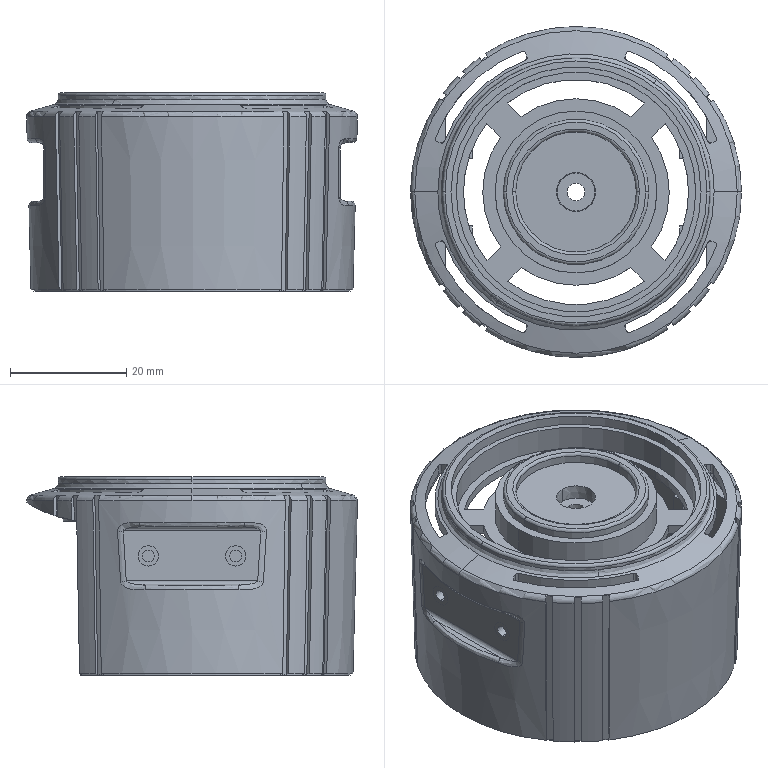Part | NX | features BREP 5 | 5 solids | 391 faces | box 56.842 x 56.842 x 34.1 mm | volume 13969 mm3 | plane 186 | cylinder 118 | cone 58 | spline 21 | torus 8 | commonest cylinder face diameters 0.8 x20 3.5 x16 6.4 x12 54.4 x10 2 x8 38.637 x6